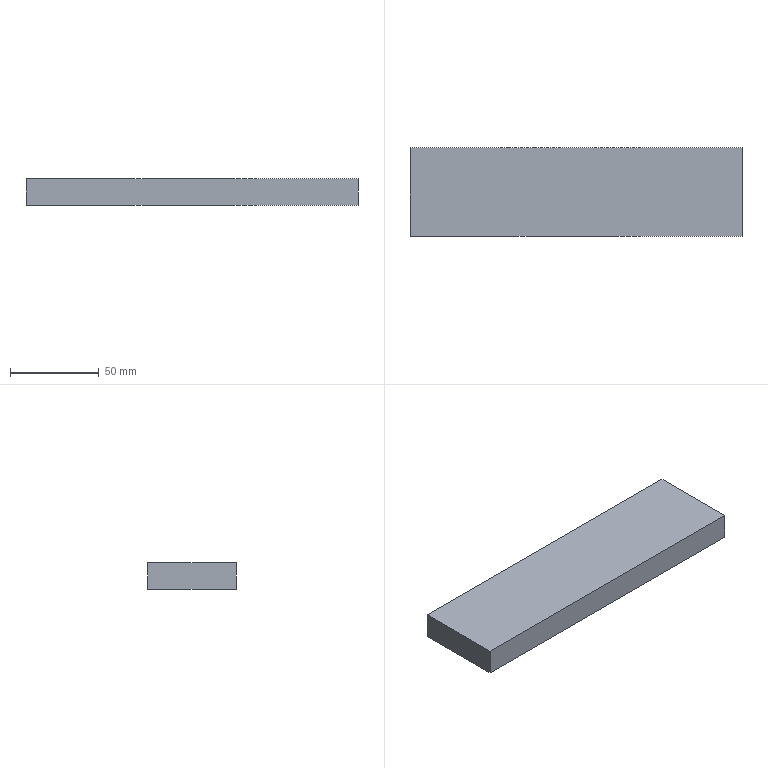Part | SolidWorks | features Extrusion 1 | 1 solid | 6 faces | box 187 x 50 x 15 mm | volume 140250 mm3 | plane 6
STEP:
#1=CARTESIAN_POINT('',(-93.5,25.,0.));
#2=VERTEX_POINT('',#1);
#3=CARTESIAN_POINT('',(-93.5,-25.,0.));
#4=VERTEX_POINT('',#3);
#5=CARTESIAN_POINT('',(-93.5,25.,0.));
#6=DIRECTION('',(0.,-1.,0.));
#7=VECTOR('',#6,1000.);
#8=LINE('',#5,#7);
#9=EDGE_CURVE('',#2,#4,#8,.T.);
#10=ORIENTED_EDGE('',*,*,#9,.T.);
#11=CARTESIAN_POINT('',(-93.5,-25.,15.));
#12=VERTEX_POINT('',#11);
#13=CARTESIAN_POINT('',(-93.5,-25.,15.));
#14=DIRECTION('',(0.,0.,-1.));
#15=VECTOR('',#14,1000.);
#16=LINE('',#13,#15);
#17=EDGE_CURVE('',#12,#4,#16,.T.);
#18=ORIENTED_EDGE('',*,*,#17,.F.);
#19=CARTESIAN_POINT('',(-93.5,25.,15.));
#20=VERTEX_POINT('',#19);
#21=CARTESIAN_POINT('',(-93.5,25.,15.));
#22=DIRECTION('',(0.,-1.,0.));
#23=VECTOR('',#22,1000.);
#24=LINE('',#21,#23);
#25=EDGE_CURVE('',#20,#12,#24,.T.);
#26=ORIENTED_EDGE('',*,*,#25,.F.);
#27=CARTESIAN_POINT('',(-93.5,25.,15.));
#28=DIRECTION('',(0.,0.,-1.));
#29=VECTOR('',#28,1000.);
#30=LINE('',#27,#29);
#31=EDGE_CURVE('',#20,#2,#30,.T.);
#32=ORIENTED_EDGE('',*,*,#31,.T.);
#33=EDGE_LOOP('',(#10,#18,#26,#32));
#34=FACE_OUTER_BOUND('',#33,.T.);
#35=CARTESIAN_POINT('',(-93.5,25.,15.));
#36=DIRECTION('',(1.,0.,0.));
#37=DIRECTION('',(0.,1.,0.));
#38=AXIS2_PLACEMENT_3D('',#35,#36,#37);
#39=PLANE('',#38);
#40=ADVANCED_FACE('',(#34),#39,.F.);
#41=CARTESIAN_POINT('',(93.5,-25.,0.));
#42=VERTEX_POINT('',#41);
#43=CARTESIAN_POINT('',(93.5,-25.,0.));
#44=DIRECTION('',(1.,0.,0.));
#45=VECTOR('',#44,1000.);
#46=LINE('',#43,#45);
#47=EDGE_CURVE('',#4,#42,#46,.T.);
#48=ORIENTED_EDGE('',*,*,#47,.T.);
#49=CARTESIAN_POINT('',(93.5,-25.,15.));
#50=VERTEX_POINT('',#49);
#51=CARTESIAN_POINT('',(93.5,-25.,15.));
#52=DIRECTION('',(0.,0.,-1.));
#53=VECTOR('',#52,1000.);
#54=LINE('',#51,#53);
#55=EDGE_CURVE('',#50,#42,#54,.T.);
#56=ORIENTED_EDGE('',*,*,#55,.F.);
#57=CARTESIAN_POINT('',(93.5,-25.,15.));
#58=DIRECTION('',(1.,0.,0.));
#59=VECTOR('',#58,1000.);
#60=LINE('',#57,#59);
#61=EDGE_CURVE('',#12,#50,#60,.T.);
#62=ORIENTED_EDGE('',*,*,#61,.F.);
#63=ORIENTED_EDGE('',*,*,#17,.T.);
#64=EDGE_LOOP('',(#48,#56,#62,#63));
#65=FACE_OUTER_BOUND('',#64,.T.);
#66=CARTESIAN_POINT('',(93.5,-25.,15.));
#67=DIRECTION('',(0.,1.,0.));
#68=DIRECTION('',(-1.,0.,0.));
#69=AXIS2_PLACEMENT_3D('',#66,#67,#68);
#70=PLANE('',#69);
#71=ADVANCED_FACE('',(#65),#70,.F.);
#72=CARTESIAN_POINT('',(93.5,25.,0.));
#73=VERTEX_POINT('',#72);
#74=CARTESIAN_POINT('',(93.5,25.,0.));
#75=DIRECTION('',(0.,1.,0.));
#76=VECTOR('',#75,1000.);
#77=LINE('',#74,#76);
#78=EDGE_CURVE('',#42,#73,#77,.T.);
#79=ORIENTED_EDGE('',*,*,#78,.T.);
#80=CARTESIAN_POINT('',(93.5,25.,15.));
#81=VERTEX_POINT('',#80);
#82=CARTESIAN_POINT('',(93.5,25.,15.));
#83=DIRECTION('',(0.,0.,-1.));
#84=VECTOR('',#83,1000.);
#85=LINE('',#82,#84);
#86=EDGE_CURVE('',#81,#73,#85,.T.);
#87=ORIENTED_EDGE('',*,*,#86,.F.);
#88=CARTESIAN_POINT('',(93.5,25.,15.));
#89=DIRECTION('',(0.,1.,0.));
#90=VECTOR('',#89,1000.);
#91=LINE('',#88,#90);
#92=EDGE_CURVE('',#50,#81,#91,.T.);
#93=ORIENTED_EDGE('',*,*,#92,.F.);
#94=ORIENTED_EDGE('',*,*,#55,.T.);
#95=EDGE_LOOP('',(#79,#87,#93,#94));
#96=FACE_OUTER_BOUND('',#95,.T.);
#97=CARTESIAN_POINT('',(93.5,25.,15.));
#98=DIRECTION('',(-1.,0.,0.));
#99=DIRECTION('',(0.,0.,1.));
#100=AXIS2_PLACEMENT_3D('',#97,#98,#99);
#101=PLANE('',#100);
#102=ADVANCED_FACE('',(#96),#101,.F.);
#103=CARTESIAN_POINT('',(93.5,25.,0.));
#104=DIRECTION('',(-1.,0.,0.));
#105=VECTOR('',#104,1000.);
#106=LINE('',#103,#105);
#107=EDGE_CURVE('',#73,#2,#106,.T.);
#108=ORIENTED_EDGE('',*,*,#107,.T.);
#109=ORIENTED_EDGE('',*,*,#31,.F.);
#110=CARTESIAN_POINT('',(93.5,25.,15.));
#111=DIRECTION('',(-1.,0.,0.));
#112=VECTOR('',#111,1000.);
#113=LINE('',#110,#112);
#114=EDGE_CURVE('',#81,#20,#113,.T.);
#115=ORIENTED_EDGE('',*,*,#114,.F.);
#116=ORIENTED_EDGE('',*,*,#86,.T.);
#117=EDGE_LOOP('',(#108,#109,#115,#116));
#118=FACE_OUTER_BOUND('',#117,.T.);
#119=CARTESIAN_POINT('',(93.5,25.,15.));
#120=DIRECTION('',(0.,-1.,0.));
#121=DIRECTION('',(1.,0.,0.));
#122=AXIS2_PLACEMENT_3D('',#119,#120,#121);
#123=PLANE('',#122);
#124=ADVANCED_FACE('',(#118),#123,.F.);
#125=ORIENTED_EDGE('',*,*,#25,.T.);
#126=ORIENTED_EDGE('',*,*,#61,.T.);
#127=ORIENTED_EDGE('',*,*,#92,.T.);
#128=ORIENTED_EDGE('',*,*,#114,.T.);
#129=EDGE_LOOP('',(#125,#126,#127,#128));
#130=FACE_OUTER_BOUND('',#129,.T.);
#131=CARTESIAN_POINT('',(0.,0.,15.));
#132=DIRECTION('',(0.,0.,-1.));
#133=DIRECTION('',(-1.,0.,0.));
#134=AXIS2_PLACEMENT_3D('',#131,#132,#133);
#135=PLANE('',#134);
#136=ADVANCED_FACE('',(#130),#135,.F.);
#137=ORIENTED_EDGE('',*,*,#9,.F.);
#138=ORIENTED_EDGE('',*,*,#107,.F.);
#139=ORIENTED_EDGE('',*,*,#78,.F.);
#140=ORIENTED_EDGE('',*,*,#47,.F.);
#141=EDGE_LOOP('',(#137,#138,#139,#140));
#142=FACE_OUTER_BOUND('',#141,.T.);
#143=CARTESIAN_POINT('',(0.,0.,0.));
#144=DIRECTION('',(0.,0.,-1.));
#145=DIRECTION('',(-1.,0.,0.));
#146=AXIS2_PLACEMENT_3D('',#143,#144,#145);
#147=PLANE('',#146);
#148=ADVANCED_FACE('',(#142),#147,.T.);
#149=CLOSED_SHELL('',(#40,#71,#102,#124,#136,#148));
#150=MANIFOLD_SOLID_BREP('',#149);
#151=CARTESIAN_POINT('',(0.,0.,0.));
#152=DIRECTION('',(0.,0.,1.));
#153=DIRECTION('',(1.,0.,0.));
#154=AXIS2_PLACEMENT_3D('',#151,#152,#153);
#155=(LENGTH_UNIT()NAMED_UNIT(*)SI_UNIT(.MILLI.,.METRE.));
#156=UNCERTAINTY_MEASURE_WITH_UNIT(LENGTH_MEASURE(0.00001),#155,'','');
#157=(NAMED_UNIT(*)PLANE_ANGLE_UNIT()SI_UNIT($,.RADIAN.));
#158=(NAMED_UNIT(*)SI_UNIT($,.STERADIAN.)SOLID_ANGLE_UNIT());
#159=(GEOMETRIC_REPRESENTATION_CONTEXT(3)GLOBAL_UNCERTAINTY_ASSIGNED_CONTEXT((#156))GLOBAL_UNIT_ASSIGNED_CONTEXT((#155,#157,#158))REPRESENTATION_CONTEXT('',''));
#160=ADVANCED_BREP_SHAPE_REPRESENTATION('',(#150,#154),#159);